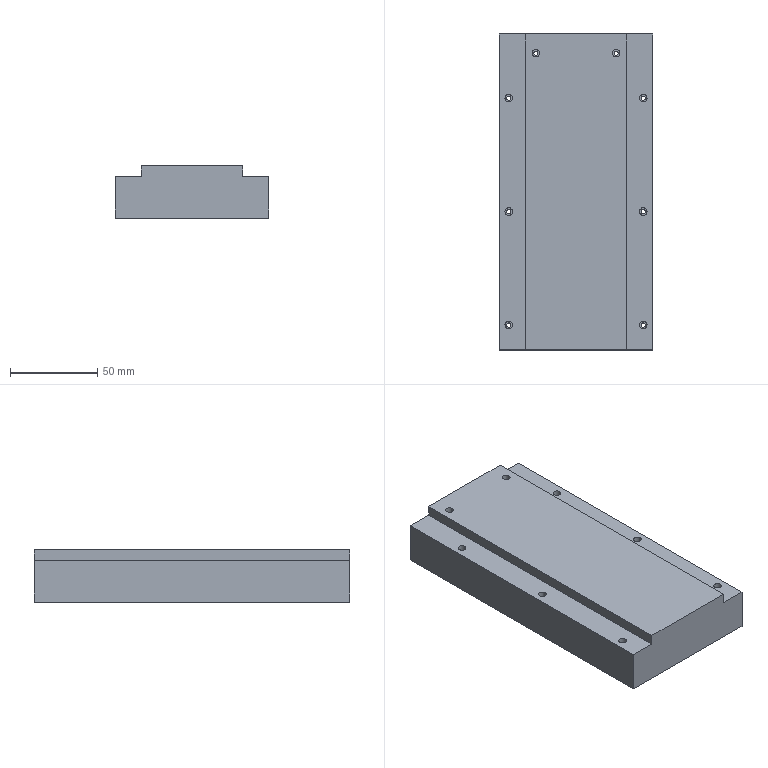NC program | NX | posted with a generic post | part box 88 x 181.05 x 30 mm
Lines 1 to 846 of 5763:
N10 G17 G21 G94 G90
(DYNAMIC_ROUGH_1 , TOOL : D12-36-D12-75-3T-ROUGH)
N12 T02 M6
N14 G54
N16 G17 G0 G90 X-53.52 Y-90.121 S6500 M3
N18 G43 Z20. H2
N20 Z-4.35
N22 G94 G1 X-53.495 Y-90.12 Z-4.506 F2500.
N24 X-53.47 Y-90.118 Z-4.568
N26 X-53.445 Y-90.117 Z-4.613
N28 X-53.42 Y-90.116 Z-4.65
N30 X-53.396 Y-90.115 Z-4.681
N32 X-53.371 Y-90.114 Z-4.707
N34 X-53.346 Y-90.113 Z-4.73
N36 X-53.321 Y-90.111 Z-4.75
N38 X-53.296 Y-90.11 Z-4.768
N40 X-53.271 Y-90.109 Z-4.783
N42 X-53.246 Y-90.108 Z-4.797
N44 X-53.221 Y-90.107 Z-4.808
N46 X-53.196 Y-90.106 Z-4.818
N48 X-53.171 Y-90.104 Z-4.827
N50 X-53.146 Y-90.103 Z-4.834
N52 X-53.121 Y-90.102 Z-4.84
N54 X-53.096 Y-90.101 Z-4.844
N56 X-53.071 Y-90.1 Z-4.847
N58 X-53.046 Y-90.098 Z-4.849
N60 X-53.021 Y-90.097 Z-4.85
N62 X-51.068 Y-90.006
N64 G3 X-50.02 Y-89.293 R1.213
N66 X-49.362 Y-86.484 R9.514
N68 X-49.037 Y-79.172 R75.262
N70 G1 X-49.001 Y-66.326
N72 X-48.999 Y87.423
N74 G2 X-47.162 Y91.584 R6.412
N76 G1 X-46.942 Y91.934
N78 X-46.004 Y93.031
N80 X-44.907 Y93.969
N82 X-43.676 Y94.723
N84 X-42.342 Y95.275
N86 X-40.938 Y95.612
N88 X-39.499 Y95.725
N90 X39.501
N92 G2 X41.712 Y95.551 R48.18
N94 X44.909 Y93.967 R6.737
N96 G1 X46.006 Y93.029
N98 X46.944 Y91.932
N100 X47.698 Y90.701
N102 X48.25 Y89.367
N104 X48.587 Y87.963
N106 G2 X48.976 Y78.131 R110.083
N108 G1 X48.999 Y65.981
N110 Y-87.347
N112 G2 X48.708 Y-89.117 R7.326
N114 X48.58 Y-90.736 R17.134
N116 G1 X48.227 Y-91.899
N118 X47.654 Y-92.971
N120 X46.883 Y-93.91
N122 X45.943 Y-94.681
N124 X44.871 Y-95.253
N126 X43.708 Y-95.606
N128 X42.499 Y-95.725
N130 X-42.501
N132 X-43.711 Y-95.605
N134 X-44.874 Y-95.252
N136 X-45.946 Y-94.679
N138 X-46.885 Y-93.908
N140 X-47.656 Y-92.968
N142 X-48.228 Y-91.896
N144 X-48.581 Y-90.733
N146 X-48.7 Y-89.525
N148 Y86.526
N150 X-48.586 Y87.965
N152 X-48.249 Y89.369
N154 X-47.697 Y90.703
N156 X-47.109 Y91.662
N158 G3 X-46.968 Y92.583 R1.202
N160 G1 X-47.118 Y93.176
N162 X-47.698 Y95.468 Z-4.75
N164 G2 X-47.663 Y96.409 R1.311 F15000.
N166 X-47.109 Y96.982 R1.205
N168 G1 X-45.901 Y97.589
N170 X-44.687 Y98.181
N172 G2 X-40.93 Y99.09 R10.745
N174 X-34.294 Y99.303 R110.869
N176 G1 X36.785 Y99.405
N178 G2 X37.775 Y98.885 R1.201
N180 G1 X37.909 Y98.691
N182 X39.25 Y96.744 Z-4.85 F2500.
N184 X39.493 Y96.387
N186 X39.748 Y96.038
N188 G3 X40.547 Y95.642 R1.203
N190 G1 X40.94 Y95.611
N192 X42.344 Y95.274
N194 X43.678 Y94.722
N196 X44.893 Y93.977
N198 X46.006 Y93.029
N200 X46.944 Y91.932
N202 X47.698 Y90.701
N204 X48.25 Y89.367
N206 X48.587 Y87.963
N208 X48.7 Y86.524
N210 Y-89.201
N212 G3 X49.538 Y-90.354 R1.212
N214 G1 X51.525 Y-90.997
N216 X51.549 Y-91.005 Z-4.849
N218 X51.572 Y-91.013 Z-4.847
N220 X51.596 Y-91.021 Z-4.844
N222 X51.62 Y-91.028 Z-4.84
N224 X51.644 Y-91.036 Z-4.834
N226 X51.667 Y-91.044 Z-4.827
N228 X51.691 Y-91.051 Z-4.818
N230 X51.715 Y-91.059 Z-4.808
N232 X51.739 Y-91.067 Z-4.797
N234 X51.763 Y-91.075 Z-4.783
N236 X51.786 Y-91.082 Z-4.768
N238 X51.81 Y-91.09 Z-4.75
N240 X51.834 Y-91.098 Z-4.73
N242 X51.858 Y-91.105 Z-4.707
N244 X51.882 Y-91.113 Z-4.681
N246 X51.905 Y-91.121 Z-4.65
N248 X51.929 Y-91.128 Z-4.613
N250 X51.953 Y-91.136 Z-4.568
N252 X51.977 Y-91.144 Z-4.506
N254 X52. Y-91.152 Z-4.35
N256 G0 Z20.
N258 X-39.874 Y-99.175
N260 Z-0.35
N262 G1 X-39.878 Y-99.15 Z-0.506
N264 X-39.881 Y-99.126 Z-0.568
N266 X-39.885 Y-99.101 Z-0.613
N268 X-39.888 Y-99.076 Z-0.65
N270 X-39.892 Y-99.051 Z-0.681
N272 X-39.895 Y-99.027 Z-0.707
N274 X-39.899 Y-99.002 Z-0.73
N276 X-39.902 Y-98.977 Z-0.75
N278 X-39.906 Y-98.952 Z-0.768
N280 X-39.909 Y-98.928 Z-0.783
N282 X-39.913 Y-98.903 Z-0.797
N284 X-39.916 Y-98.878 Z-0.808
N286 X-39.92 Y-98.853 Z-0.818
N288 X-39.923 Y-98.829 Z-0.827
N290 X-39.927 Y-98.804 Z-0.834
N292 X-39.93 Y-98.779 Z-0.84
N294 X-39.934 Y-98.754 Z-0.844
N296 X-39.937 Y-98.73 Z-0.847
N298 X-39.941 Y-98.705 Z-0.849
N300 X-39.944 Y-98.68 Z-0.85
N302 X-40.222 Y-96.709
N304 G3 X-41.288 Y-95.674 R1.212
N306 G1 X-42.033 Y-95.591
N308 X-43.182 Y-95.228
N310 X-44.239 Y-94.65
N312 X-45.165 Y-93.878
N314 X-45.923 Y-92.942
N316 X-46.487 Y-91.877
N318 G2 X-47.288 Y-87.904 R17.526
N320 X-47.643 Y-79.515 R88.902
N322 G1 X-47.674 Y-66.465
N324 X-47.672 Y83.61
N326 G2 X-46.746 Y88.508 R11.663
N328 X-42.239 Y92.861 R8.861
N330 X-36.88 Y94.258 R18.044
N332 X-29.244 Y94.656 R73.074
N334 X-16.645 Y94.699 R816.574
N336 G1 X36.605 Y94.697
N338 G2 X41.502 Y93.762 R11.592
N340 X45.835 Y89.266 R8.86
N342 X47.231 Y83.917 R18.017
N344 X47.625 Y76.506 R70.519
N346 X47.674 Y61.956 R900.28
N348 G1 X47.672 Y-86.457
N350 G2 X47.01 Y-89.127 R6.226
N352 G3 X46.832 Y-90.726 R13.646
N354 G1 X46.485 Y-91.879
N356 X45.922 Y-92.944
N358 X45.163 Y-93.88
N360 X44.237 Y-94.651
N362 X43.18 Y-95.229
N364 X42.031 Y-95.591
N366 X41.285 Y-95.674
N368 X42.031 Y-95.591
N370 X43.18 Y-95.229
N372 X44.237 Y-94.651
N374 X45.163 Y-93.88
N376 X45.922 Y-92.944
N378 X46.485 Y-91.879
N380 X46.832 Y-90.726
N382 G3 X47.025 Y-86.809 R36.858
N384 X47.074 Y-74.809 R770.028
N386 G1 Y72.941
N388 G3 X46.773 Y81.873 R128.023
N390 X45.657 Y87.368 R20.478
N392 X39.826 Y92.921 R9.356
N394 X34.457 Y93.903 R20.366
N396 X25.911 Y94.093 R139.133
N398 G1 X20.061 Y94.099
N400 X-20.589 Y94.097
N402 G3 X-32.737 Y93.94 R292.698
N404 X-38.9 Y93.143 R30.596
N406 X-43.759 Y90.43 R9.942
N408 X-46.29 Y85.542 R10.716
N410 X-46.977 Y79.592 R29.521
N412 X-47.074 Y65.793 R491.248
N414 G1 X-47.069 Y-83.686
N416 X-46.95 Y-85.017
N418 Y-89.525
N420 X-46.833 Y-90.723
N422 X-46.95 Y-89.525
N424 Y78.226
N426 X-46.846 Y79.678
N428 G2 X-46.158 Y82.346 R22.208
N430 X-44.732 Y86.292 R19.015
N432 X-39.573 Y90.969 R10.862
N434 X-33.433 Y92.587 R20.925
N436 X-25.049 Y93.048 R78.213
N438 X-11.175 Y93.098 R856.081
N440 G1 X22.65 Y93.097
N442 G2 X32.773 Y92.938 R194.218
N444 X37.866 Y92.105 R20.135
N446 X43.556 Y87.209 R10.042
N448 X44.657 Y84.663 R19.301
N450 G1 X45.331 Y83.739
N452 X46.029 Y82.461
N454 X46.537 Y81.098
N456 X46.846 Y79.676
N458 X46.95 Y78.224
N460 X46.961 Y-89.466
N462 X47.375 Y-91.26
N464 G3 X49.753 Y-91.157 R1.212
N466 G1 X49.757 Y-91.132 Z-0.849
N468 X49.76 Y-91.107 Z-0.847
N470 X49.764 Y-91.083 Z-0.844
N472 X49.768 Y-91.058 Z-0.84
N474 X49.771 Y-91.033 Z-0.834
N476 X49.775 Y-91.008 Z-0.827
N478 X49.779 Y-90.984 Z-0.818
N480 X49.782 Y-90.959 Z-0.808
N482 X49.786 Y-90.934 Z-0.797
N484 X49.79 Y-90.909 Z-0.783
N486 X49.793 Y-90.885 Z-0.768
N488 X49.797 Y-90.86 Z-0.75
N490 X49.8 Y-90.835 Z-0.73
N492 X49.804 Y-90.811 Z-0.707
N494 X49.808 Y-90.786 Z-0.681
N496 X49.811 Y-90.761 Z-0.65
N498 X49.815 Y-90.736 Z-0.613
N500 X49.819 Y-90.712 Z-0.568
N502 X49.822 Y-90.687 Z-0.506
N504 X49.826 Y-90.662 Z-0.35
N506 G0 Z20.
N508 X-49.94 Y78.855
N510 Z-0.35
N512 G1 X-49.935 Y78.879 Z-0.506
N514 X-49.929 Y78.904 Z-0.568
N516 X-49.924 Y78.928 Z-0.613
N518 X-49.919 Y78.952 Z-0.65
N520 X-49.913 Y78.977 Z-0.681
N522 X-49.908 Y79.001 Z-0.707
N524 X-49.903 Y79.026 Z-0.73
N526 X-49.897 Y79.05 Z-0.75
N528 X-49.892 Y79.075 Z-0.768
N530 X-49.887 Y79.099 Z-0.783
N532 X-49.881 Y79.123 Z-0.797
N534 X-49.876 Y79.148 Z-0.808
N536 X-49.871 Y79.172 Z-0.818
N538 X-49.865 Y79.197 Z-0.827
N540 X-49.86 Y79.221 Z-0.834
N542 X-49.855 Y79.246 Z-0.84
N544 X-49.849 Y79.27 Z-0.844
N546 X-49.844 Y79.294 Z-0.847
N548 X-49.839 Y79.319 Z-0.849
N550 X-49.833 Y79.343 Z-0.85
N552 G2 X-48.807 Y80.286 R1.212
N554 G1 X-47.462 Y80.462
N556 G3 X-46.484 Y81.24 R1.213
N558 G2 X-44.862 Y84.426 R11.149
N560 X-36.944 Y90.363 R15.136
N562 X-29.74 Y91.732 R30.415
N564 X-19.024 Y92.078 R141.649
N566 G1 X-8.299 Y92.098
N568 X22.151 Y92.096
N570 G2 X31.673 Y91.933 R170.459
N572 X36.166 Y91.149 R16.744
N574 X41.207 Y87.465 R11.157
N576 G1 X41.492 Y87.228
N578 X42.265 Y86.805
N580 X43.43 Y85.933
N582 X44.459 Y84.904
N584 X44.729 Y84.543
N586 X44.459 Y84.904
N588 X43.43 Y85.933
N590 X42.265 Y86.805
N592 G2 X39.863 Y88.308 R17.315
N594 G3 X32.756 Y90.978 R16.566
N596 X25.502 Y91.452 R55.845
N598 X14.177 Y91.498 R749.014
N600 G1 X-11.773 Y91.496
N602 G3 X-26.246 Y91.32 R365.365
N604 X-33.983 Y90.418 R44.319
N606 X-40.322 Y87.751 R18.323
N608 G1 X-40.986 Y87.504
N610 X-42.264 Y86.806
N612 X-43.429 Y85.934
N614 X-44.458 Y84.905
N616 X-45.33 Y83.74
N618 X-44.458 Y84.905
N620 X-43.429 Y85.934
N622 X-42.264 Y86.806
N624 X-40.986 Y87.504
N626 X-39.623 Y88.012
N628 G3 X-34.961 Y89.111 R234.037
N630 G2 X-24.545 Y90.316 R59.221
N632 X-8.797 Y90.495 R437.922
N634 G1 X15.128 Y90.497
N636 G2 X27.576 Y90.356 R308.726
N638 X33.881 Y89.505 R29.282
N640 X36.844 Y88.436 R28.311
N642 G1 X38.203 Y88.321
N644 X39.625 Y88.011
N646 X40.988 Y87.503
N648 X41.317 Y87.323
N650 X40.988 Y87.503
N652 X39.625 Y88.011
N654 X38.203 Y88.321
N656 G2 X34.365 Y88.85 R21.203
N658 G3 X24.75 Y89.805 R56.039
N660 X10.201 Y89.897 R645.563
N662 G1 X-31.401
N664 X-31.561 Y89.907
N666 X-34.544 Y90.31
N668 X-35.502 Y90.445 Z-0.809
N670 G2 X-36.436 Y91.374 Z-0.75 R1.199
N672 X-36.008 Y92.557 R1.201 F15000.
N674 G1 X-35.708 Y92.793
N676 X-35.418 Y93.041
N678 G3 X-37.378 Y94.369 R-1.2
N680 G1 X-38.819 Y91.233
N682 X-39.403 Y89.951 Z-0.81 F2500.
N684 G3 X-39.379 Y89.022 Z-0.85 R1.2
N686 X-38.201 Y88.321 R1.2
N688 G2 X-35.308 Y88.441 R34.792
N690 X-24.995 Y88.872 R111.399
N692 G1 X-12.695 Y88.896
N694 X30.651 Y88.891
N696 X32.367 Y88.433
N698 X36.751 Y88.425
N700 X-35.658
N702 G2 X-36.869 Y89.578 R1.212
N704 G1 X-36.956 Y91.373
N706 X-36.957 Y91.398 Z-0.849
N708 X-36.958 Y91.423 Z-0.847
N710 X-36.959 Y91.448 Z-0.844
N712 X-36.961 Y91.473 Z-0.84
N714 X-36.962 Y91.498 Z-0.834
N716 X-36.963 Y91.523 Z-0.827
N718 X-36.964 Y91.548 Z-0.818
N720 X-36.965 Y91.573 Z-0.808
N722 X-36.967 Y91.598 Z-0.797
N724 X-36.968 Y91.623 Z-0.783
N726 X-36.969 Y91.648 Z-0.768
N728 X-36.97 Y91.673 Z-0.75
N730 X-36.971 Y91.698 Z-0.73
N732 X-36.973 Y91.723 Z-0.707
N734 X-36.974 Y91.748 Z-0.681
N736 X-36.975 Y91.773 Z-0.65
N738 X-36.976 Y91.798 Z-0.613
N740 X-36.978 Y91.823 Z-0.568
N742 X-36.979 Y91.848 Z-0.506
N744 X-36.98 Y91.873 Z-0.35
N746 G0 Z20.
N748 X-50.473 Y-71.29
N750 Z0.65
N752 G1 X-50.448 Y-71.289 Z0.494
N754 X-50.423 Y-71.288 Z0.432
N756 X-50.398 Y-71.287 Z0.387
N758 X-50.373 Y-71.286 Z0.35
N760 X-50.348 Y-71.285 Z0.319
N762 X-50.323 Y-71.284 Z0.293
N764 X-50.298 Y-71.283 Z0.27
N766 X-50.273 Y-71.282 Z0.25
N768 X-50.248 Y-71.281 Z0.232
N770 X-50.223 Y-71.28 Z0.217
N772 X-50.198 Y-71.279 Z0.203
N774 X-50.173 Y-71.278 Z0.192
N776 X-50.148 Y-71.277 Z0.182
N778 X-50.123 Y-71.276 Z0.173
N780 X-50.098 Y-71.274 Z0.166
N782 X-50.073 Y-71.273 Z0.16
N784 X-50.048 Y-71.272 Z0.156
N786 X-50.023 Y-71.271 Z0.153
N788 X-49.998 Y-71.27 Z0.151
N790 X-49.973 Y-71.269 Z0.15
N792 X-48.031 Y-71.187
N794 G3 X-46.973 Y-70.465 R1.213
N796 X-46.302 Y-67.553 R9.948
N798 X-45.979 Y-59.784 R82.298
N800 G1 X-45.95 Y-48.577
N802 X-45.949 Y75.248
N804 G2 X-45.106 Y80.397 R13.708
N806 X-39.317 Y85.941 R9.705
N808 X-33.68 Y87.109 R21.372
N810 X-24.387 Y87.409 R116.295
N812 G1 X-14.562 Y87.424
N814 X33.813 Y87.423
N816 G2 X39.028 Y86.538 R13.516
N818 X44.42 Y80.885 R9.649
N820 X45.625 Y75.178 R21.222
N822 X45.932 Y66.036 R112.653
N824 G1 X45.949 Y56.211
N826 Y-86.401
N828 G2 X43.996 Y-90.89 R6.382
N830 X39.218 Y-93.589 R10.942
N832 X33.152 Y-94.516 R27.573
N834 X21.905 Y-94.72 R209.141
N836 G1 X15.83 Y-94.724
N838 X-37.701 Y-94.723
N840 G2 X-42.115 Y-92.77 R6.387
N842 X-44.814 Y-87.993 R10.942
N844 X-45.741 Y-81.927 R27.572
N846 X-45.897 Y-73.531 R100.324
N848 X-45.346 Y-67.739 R373.993
N850 G3 X-44.978 Y-57.314 R145.466
N852 G1 X-44.951 Y-45.802
N854 X-44.95 Y72.773
N856 G2 X-44.478 Y77.461 R18.378
N858 X-39.588 Y83.685 R10.162
N860 X-33.653 Y85.699 R17.722
N862 X-26.035 Y86.326 R54.495
N864 X-10.361 Y86.424 R698.175
N866 G1 X31.322 Y86.423
N868 G2 X35.936 Y85.967 R18.462
N870 X42.171 Y81.119 R10.142
N872 X44.209 Y75.184 R17.634
N874 X44.854 Y67.343 R54.779
N876 X44.949 Y51.668 R715.077
N878 G1 X44.947 Y-83.321
N880 G2 X41.585 Y-90.007 R8.753
N882 X36.039 Y-92.634 R14.146
N884 X29.058 Y-93.536 R36.57
N886 X17.285 Y-93.719 R264.984
N888 G1 X10.685 Y-93.724
N890 X-34.547 Y-93.722
N892 G2 X-41.232 Y-90.359 R8.754
N894 X-43.859 Y-84.813 R14.146
N896 X-44.765 Y-77.758 R36.7
N898 X-44.578 Y-70.94 R54.381
N900 G3 X-43.974 Y-55.148 R201.941
N902 G1 X-43.951 Y-45.126
N904 X-43.95 Y70.373
N906 G2 X-43.625 Y75.004 R23.77
N908 X-38.443 Y82.246 R11.011
N910 X-32.202 Y84.531 R18.421
N912 X-24.221 Y85.292 R51.99
N914 X-9.672 Y85.422 R497.651
N916 G1 X28.697 Y85.423
N918 G2 X33.258 Y85.152 R26.312
N920 X40.706 Y80.013 R10.988
N922 X43.059 Y73.644 R18.365
N924 X43.822 Y65.513 R52.991
N926 X43.947 Y51.49 R498.44
N928 G1 X43.949 Y-80.135
N930 G2 X42.608 Y-85.754 R10.725
N932 X37.516 Y-90.3 R11.576
N934 X31.183 Y-92.092 R21.534
N936 X22.657 Y-92.651 R71.992
N938 X7.582 Y-92.723 R841.331
N940 G1 X-31.568 Y-92.722
N942 G2 X-40.623 Y-87.881 R10.362
N944 X-42.973 Y-81.908 R17.246
N946 X-43.599 Y-73.326 R35.962
N948 X-43.178 Y-64.218 R994.69
N950 G3 X-42.953 Y-46.924 R477.344
N952 G1 X-42.951 Y-41.977
N954 Y68.198
N956 G2 X-42.693 Y72.836 R28.899
N958 X-37.107 Y81.028 R11.754
N960 X-30.594 Y83.448 R19.399
N962 X-22.394 Y84.269 R52.819
N964 X-7.92 Y84.421 R439.798
N966 G1 X26.522 Y84.423
N968 G2 X31.31 Y84.175 R30.503
N970 X39.557 Y78.569 R11.768
N972 X41.973 Y72.05 R19.492
N974 X42.786 Y64.075 R52.152
N976 X42.947 Y48.776 R441.27
N978 G1 X42.948 Y-77.472
N980 G2 X42.372 Y-82.141 R14.981
N982 X37.216 Y-88.477 R11.471
N984 X30.666 Y-90.818 R19.57
N986 X22.534 Y-91.583 R55.009
N988 X5.961 Y-91.722 R556.884
N990 G1 X-28.697 Y-91.723
N992 G2 X-33.366 Y-91.147 R14.987
N994 X-39.662 Y-86.054 R11.444
N996 X-42.077 Y-79.001 R18.872
N998 X-42.426 Y-71.293 R44.811
N1000 G3 X-42.016 Y-57.064 R810.514
N1002 X-41.952 Y-41.976 R884.905
N1004 G1 X-41.951 Y66.024
N1006 G2 X-41.69 Y71.112 R32.993
N1008 X-35.661 Y79.952 R12.421
N1010 X-28.85 Y82.427 R20.644
N1012 X-20.274 Y83.267 R56.556
N1014 X-5.276 Y83.421 R468.655
N1016 G1 X24.649 Y83.422
N1018 G2 X29.662 Y83.158 R31.967
N1020 X38.453 Y77.168 R12.413
N1022 X40.945 Y70.35 R20.58
N1024 X41.785 Y61.925 R55.657
N1026 X41.946 Y46.627 R453.996
N1028 G1 X41.948 Y-74.922
N1030 G2 X41.546 Y-79.693 R20.631
N1032 X36.053 Y-87.19 R12.024
N1034 X29.337 Y-89.703 R19.939
N1036 X21.214 Y-90.547 R52.939
N1038 X5.541 Y-90.721 R431.809
N1040 G1 X-26.147 Y-90.722
N1042 G2 X-30.918 Y-90.321 R20.636
N1044 X-38.53 Y-84.632 R12.041
N1046 X-40.874 Y-77.789 R18.878
N1048 X-41.305 Y-70.01 R47.459
N1050 G1 X-41.069 Y-59.811
N1052 G3 X-40.952 Y-39.802 R947.688
N1054 G1 Y63.773
N1056 G2 X-40.731 Y69.165 R41.405
N1058 X-34.275 Y78.89 R13.002
N1060 X-27.462 Y81.361 R21.414
N1062 X-18.891 Y82.242 R56.151
N1064 X-2.768 Y82.421 R449.656
N1066 G1 X21.947 Y82.422
N1068 G2 X27.415 Y82.237 R47.715
N1070 X37.472 Y75.647 R13.036
N1072 X39.906 Y68.827 R21.63
N1074 X40.769 Y60.329 R56.898
N1076 X40.945 Y44.581 R441.957
N1078 G1 X40.947 Y-72.747
N1080 G2 X40.622 Y-77.603 R25.932
N1082 X34.748 Y-86.052 R12.589
N1084 X28.108 Y-88.593 R20.365
N1086 X19.844 Y-89.518 R51.656
N1088 X5.372 Y-89.718 R353.688
N1090 G1 X-0.403 Y-89.722
N1092 X-24.422 Y-89.72
N1094 G2 X-29.415 Y-89.272 R21.916
N1096 X-37.495 Y-83.107 R12.519
N1098 X-39.743 Y-76.231 R19.798
N1100 X-40.203 Y-68.077 R53.087
N1102 G1 X-40.021 Y-56.545
N1104 G3 X-39.953 Y-40.026 R952.652
N1106 G1 X-39.951 Y62.499
N1108 G2 X-39.661 Y68.035 R36.766
N1110 X-32.974 Y77.815 R13.457
N1112 X-25.865 Y80.355 R22.301
N1114 X-17.068 Y81.241 R59.092
N1116 X-1.695 Y81.419 R435.666
N1118 G1 X3.255 Y81.421
N1120 X20.897
N1122 G2 X26.435 Y81.151 R38.499
N1124 X36.343 Y74.437 R13.463
N1126 X38.867 Y67.398 R22.255
N1128 X39.76 Y58.677 R58.261
N1130 X39.945 Y42.554 R443.412
N1132 G1 X39.947 Y-70.021
N1134 G2 X39.74 Y-75.188 R40.472
N1136 X33.198 Y-85.11 R13.186
N1138 X26.241 Y-87.637 R21.815
N1140 X17.446 Y-88.539 R57.562
N1142 X3.348 Y-88.718 R395.952
N1144 G1 X-2.427 Y-88.721
N1146 X-22.077
N1148 G2 X-27.308 Y-88.372 R28.584
N1150 X-36.426 Y-81.679 R12.916
N1152 X-38.643 Y-74.632 R20.942
N1154 X-39.126 Y-66.403 R57.843
N1156 X-38.997 Y-53.939 R984.734
N1158 G1 X-38.953 Y-39.126
N1160 X-38.952 Y60.399
N1162 G2 X-38.709 Y66.165 R45.497
N1164 X-31.704 Y76.751 R13.906
N1166 X-24.602 Y79.299 R22.819
N1168 X-15.809 Y80.22 R58.759
N1170 X-1.636 Y80.416 R372.574
N1172 G1 X4.964 Y80.421
N1174 X19.022
N1176 G2 X24.787 Y80.166 R43.509
N1178 X35.324 Y73.091 R13.917
N1180 X37.828 Y66.047 R22.919
N1182 X38.749 Y57.178 R59.156
N1184 X38.942 Y43.005 R380.641
N1186 G1 X38.946 Y36.405
N1188 X38.945 Y-68.922
N1190 G2 X38.632 Y-74.306 R33.552
N1192 X32.068 Y-83.947 R13.575
N1194 X25.071 Y-86.554 R21.996
N1196 X16.282 Y-87.512 R56.163
N1198 X2.184 Y-87.716 R354.429
N1200 G1 X-3.591 Y-87.72
N1202 X-20.147
N1204 G2 X-25.531 Y-87.406 R33.523
N1206 X-35.333 Y-80.333 R13.274
N1208 X-37.517 Y-73.352 R21.747
N1210 X-38.061 Y-64.826 R60.003
N1212 X-37.987 Y-52.223 R857.814
N1214 G1 X-37.954 Y-37.402
N1216 X-37.953 Y58.373
N1218 G2 X-37.728 Y64.516 R53.811
N1220 X-34.575 Y72.253 R14.57
N1222 X-28.009 Y76.889 R16.251
N1224 X-20.298 Y78.742 R30.774
N1226 X-9.821 Y79.344 R102.071
N1228 X5.929 Y79.42 R875.464
N1230 G1 X17.972 Y79.419
N1232 G2 X23.807 Y79.091 R38.556
N1234 X34.226 Y71.922 R14.243
N1236 X36.819 Y64.601 R23.532
N1238 X37.758 Y55.282 R62.327
N1240 X37.944 Y38.709 R471.413
N1242 G1 X37.945 Y-66.297
N1244 G2 X37.713 Y-72.213 R48.686
N1246 X30.504 Y-83.069 R14.081
N1248 X23.235 Y-85.618 R23.469
N1250 X14.214 Y-86.528 R61.599
N1252 X-2.434 Y-86.718 R461.048
N1254 G1 X-17.372 Y-86.72
N1256 G2 X-23.289 Y-86.506 R50.75
N1258 X-30.805 Y-83.386 R13.914
N1260 X-35.231 Y-76.78 R15.43
N1262 X-36.752 Y-69.229 R29.596
N1264 X-37.025 Y-59.936 R110.162
N1266 G1 X-36.967 Y-47.214
N1268 X-36.954 Y-37.326
N1270 X-36.953 Y56.499
N1272 G2 X-36.749 Y62.867 R62.359
N1274 X-34.29 Y70.029 R15.51
N1276 X-33.206 Y71.47 R66.263
N1278 X-31.623 Y73.394 R4.42
N1280 X-23.179 Y77.011 R23.556
N1282 X-14.261 Y78.137 R53.601
N1284 X-0.09 Y78.411 R283.411
N1286 G1 X7.335 Y78.42
N1288 G2 X19.171 Y78.37 R500.313
N1290 X25.151 Y77.427 R21.045
N1292 X31.237 Y73.431 R14.644
N1294 G1 X31.716 Y73.124
N1296 G2 X32.826 Y71.733 R4.654
N1298 X35.779 Y63.513 R25.838
N1300 X36.74 Y54.121 R64.046
N1302 X36.94 Y39.648 R389.782
N1304 G1 X36.945 Y32.223
N1306 X36.943 Y-65.052
N1308 G2 X36.68 Y-70.967 R46.477
N1310 X29.387 Y-81.95 R14.418
N1312 X22.057 Y-84.562 R23.698
N1314 X12.889 Y-85.514 R61.278
N1316 X-1.284 Y-85.714 R377.233
N1318 G1 X-7.059 Y-85.719
N1320 G2 X-19.172 Y-85.684 R636.222
N1322 X-25.014 Y-84.828 R21.019
N1324 X-33.01 Y-78.028 R13.831
N1326 X-34.694 Y-73.784 R22.505
N1328 G3 X-34.949 Y-73.416 R3.436
N1330 X-35.833 Y-73.073 R1.202
N1332 G1 X-36.489 Y-73.096
N1334 X-38.853 Y-73.182 Z0.25
N1336 G2 X-40.088 Y-72.039 R1.2 F15000.
N1338 G1 X-40.262 Y-68.424
N1340 X-40.422 Y-64.808
N1342 G2 X-40.583 Y-56.539 R224.547
N1344 G1 X-40.671 Y58.179
N1346 G2 X-39.4 Y68.169 R40.678
N1348 G1 X-38.935 Y69.888
N1350 X-38.458 Y71.604
N1352 G2 X-37.578 Y72.451 R1.201
N1354 G1 X-35.832 Y72.864
N1356 X-34.473 Y73.18 Z0.191 F2500.
N1358 G2 X-33.556 Y72.964 Z0.15 R1.2
N1360 X-33.138 Y71.604 R1.2
N1362 X-34.316 Y68.921 R47.916
N1364 G3 X-36.146 Y60.918 R23.998
N1366 X-36.35 Y51.472 R146.103
N1368 G1 X-36.354 Y46.522
N1370 X-36.356 Y-40.961
N1372 X-36.397 Y-53.688
N1374 X-36.428 Y-58.103
N1376 G3 X-36.5 Y-58.808 R11.478
N1378 G1 Y-70.525
N1380 X-36.381 Y-71.431
N1382 X-36.031 Y-72.275
N1384 X-35.475 Y-73.
N1386 X-34.824 Y-73.507
N1388 G2 X-33.551 Y-75.723 R16.688
N1390 G3 X-30.151 Y-80.559 R19.286
N1392 X-22.564 Y-84.465 R14.578
N1394 X-15.999 Y-85.057 R38.168
N1396 X10.024 Y-84.997 R840.959
N1398 X19.816 Y-84.265 R81.212
N1400 X27.223 Y-82.168 R27.051
N1402 X33.816 Y-76.395 R14.827
N1404 X35.18 Y-73.393 R16.072
N1406 G1 X35.388 Y-73.083
N1408 G2 X36.774 Y-72.848 R1.2
N1410 X37.44 Y-73.774 Z0.2 R1.25
N1412 G1 X37.7 Y-74.923 Z0.25
N1414 X38.145 Y-76.889 F15000.
N1416 G2 X38.048 Y-77.69 R1.205
N1418 G1 X37.818 Y-78.152
N1420 X37.578 Y-78.608
N1422 G2 X36.843 Y-79.512 R4.064
N1424 G1 X35.756 Y-80.512
N1426 X34.646 Y-81.486
N1428 G2 X31.061 Y-84.073 R29.213
N1430 X27.091 Y-85.994 R25.672
N1432 X22.871 Y-87.296 R29.885
N1434 X19.964 Y-87.763 R25.005
N1436 G1 X17.393 Y-88.02
N1438 X14.818 Y-88.243
N1440 G2 X8.921 Y-88.547 R124.281
N1442 G1 X-6.593 Y-88.973
N1444 G2 X-19.852 Y-88.432 R97.392
N1446 G1 X-23.525 Y-88.03
N1448 G2 X-28.957 Y-86.115 R12.639
N1450 X-33.337 Y-82.259 R19.097
N1452 G1 X-34.283 Y-81.126
N1454 X-35.219 Y-79.985
N1456 X-36.316 Y-78.55
N1458 G2 X-36.554 Y-77.935 R1.211
N1460 G1 X-36.748 Y-75.768
N1462 X-36.867 Y-74.395 Z0.192 F2500.
N1464 G2 X-36.51 Y-73.506 Z0.15 R1.2
N1466 X-34.939 Y-73.411 R1.2
N1468 X-33.656 Y-74.855 R6.054
N1470 G3 X-31. Y-78.486 R43.846
N1472 X-22.543 Y-83.561 R15.621
N1474 X-15.554 Y-84.395 R36.016
N1476 X-1.531 Y-84.512 R395.884
N1478 X13.241 Y-84.252 R304.127
N1480 X21.864 Y-83.182 R51.396
N1482 X28.577 Y-80.465 R20.432
N1484 X33.249 Y-75.445 R14.48
N1486 G2 X34.272 Y-73.856 R11.957
N1488 G1 X34.445 Y-73.712
N1490 G2 X35.945 Y-73.827 R1.2
N1492 X36.318 Y-74.867 Z0.198 R1.247
N1494 G1 X36.262 Y-76.085 Z0.25
N1496 X36.173 Y-78.057 F15000.
N1498 G2 X35.823 Y-78.851 R1.203
N1500 G1 X32.687 Y-81.986
N1502 G2 X27.725 Y-85.056 R12.983
N1504 G1 X25.528 Y-85.797
N1506 G2 X19.883 Y-87.057 R35.643
N1508 X11.082 Y-88.089 R128.583
N1510 X0.76 Y-88.422 R88.684
N1512 G1 X-17.707 Y-87.941
N1514 G2 X-23.516 Y-87.095 R24.801
N1516 X-26.028 Y-86.318 R24.075
N1518 X-31.412 Y-83.109 R17.891
N1520 G1 X-31.879 Y-82.686
N1522 X-36.127 Y-78.695
N1524 G2 X-36.505 Y-77.859 R1.203
N1526 G1 X-36.568 Y-75.906
N1528 X-36.608 Y-74.521 Z0.191 F2500.
N1530 G2 X-36.205 Y-73.659 Z0.15 R1.2
N1532 X-34.75 Y-73.556 R1.2
N1534 X-33.014 Y-75.162 R7.187
N1536 G3 X-29.88 Y-78.633 R39.757
N1538 X-21.498 Y-82.937 R17.658
N1540 X-14.132 Y-83.781 R41.197
N1542 X0.567 Y-83.905 R385.48
N1544 X13.911 Y-83.583 R223.889
N1546 X22.208 Y-82.361 R43.759
N1548 X28.792 Y-79.212 R17.897
N1550 X32.216 Y-75.53 R19.693
N1552 G2 X33.456 Y-74.11 R9.423
N1554 G1 X33.649 Y-73.995
N1556 G2 X34.97 Y-74.212 R1.2
N1558 X35.353 Y-75.136 Z0.193 R1.259
N1560 G1 X35.421 Y-76.47 Z0.25
N1562 X35.505 Y-78.113 F15000.
N1564 G2 X35.026 Y-79.135 R1.201
N1566 G1 X31.476 Y-81.797
N1568 G2 X25.68 Y-84.909 R21.964
N1570 X20.711 Y-86.227 R28.796
N1572 X12.654 Y-87.095 R55.503
N1574 G1 X3.052 Y-87.401
N1576 G2 X-9.506 Y-87.719 R888.409
N1578 X-19.767 Y-86.898 R51.977
N1580 G1 X-21.22 Y-86.638
N1582 X-22.669 Y-86.361
N1584 G2 X-28.056 Y-84.459 R22.34
N1586 X-32.287 Y-81.359 R16.774
N1588 G1 X-34.75 Y-78.877
N1590 G2 X-35.016 Y-78.467 R1.249
N1592 G1 X-35.856 Y-76.31
N1594 X-36.35 Y-75.028 Z0.192 F2500.
N1596 G2 X-36.252 Y-74.072 Z0.15 R1.2
N1598 X-34.75 Y-73.556 R1.2
N1600 X-32.886 Y-74.833 R5.623
N1602 G3 X-29.64 Y-77.928 R91.293
N1604 X-20.461 Y-82.343 R20.
N1606 X-12.415 Y-83.189 R47.583
N1608 X10.981 Y-83.117 R410.702
N1610 X19.776 Y-82.201 R58.213
N1612 X26.369 Y-79.805 R20.548
N1614 X30.51 Y-76.34 R19.215
N1616 G2 X32.755 Y-74.166 R18.145
N1618 G1 X32.957 Y-74.067
N1620 G2 X34.403 Y-74.611 R1.2
N1622 X34.448 Y-75.709 Z0.198 R1.248
N1624 G1 X34.033 Y-76.862 Z0.25
N1626 X33.307 Y-78.881 F15000.
N1628 G2 X32.957 Y-79.387 R1.215
N1630 G1 X32.173 Y-80.056
N1632 X31.383 Y-80.718
N1634 G2 X29.45 Y-82.055 R17.617
N1636 G1 X27.544 Y-83.179
N1638 G2 X25.125 Y-84.376 R25.626
N1640 X22.792 Y-85.11 R13.836
N1642 G1 X21.247 Y-85.448
N1644 X19.696 Y-85.752
N1646 G2 X15.517 Y-86.261 R40.406
N1648 G1 X12.016 Y-86.504
N1650 X8.514 Y-86.733
N1652 G2 X0.028 Y-87.04 R171.983
N1654 X-4.401 Y-86.991 R130.31
N1656 G1 X-15.483 Y-86.667
N1658 G2 X-21.322 Y-85.935 R30.919
N1660 X-24.467 Y-85.077 R25.001
N1662 X-30.038 Y-82.15 R22.556
N1664 G1 X-34.404 Y-79.02
N1666 G2 X-34.834 Y-78.449 R1.208
N1668 G1 X-35.554 Y-76.437
N1670 X-36.014 Y-75.14 Z0.192 F2500.
N1672 G2 X-35.89 Y-74.188 Z0.15 R1.2
N1674 X-34.404 Y-73.7 R1.2
N1676 X-31.928 Y-75.234 R8.26
N1678 G3 X-27.88 Y-78.401 R47.571
N1680 X-18.754 Y-81.892 R23.382
N1682 X-10.092 Y-82.62 R60.584
N1684 X10.455 Y-82.52 R378.716
N1686 X19.101 Y-81.627 R57.693
N1688 X26.206 Y-78.887 R19.857
N1690 X30.104 Y-75.715 R29.623